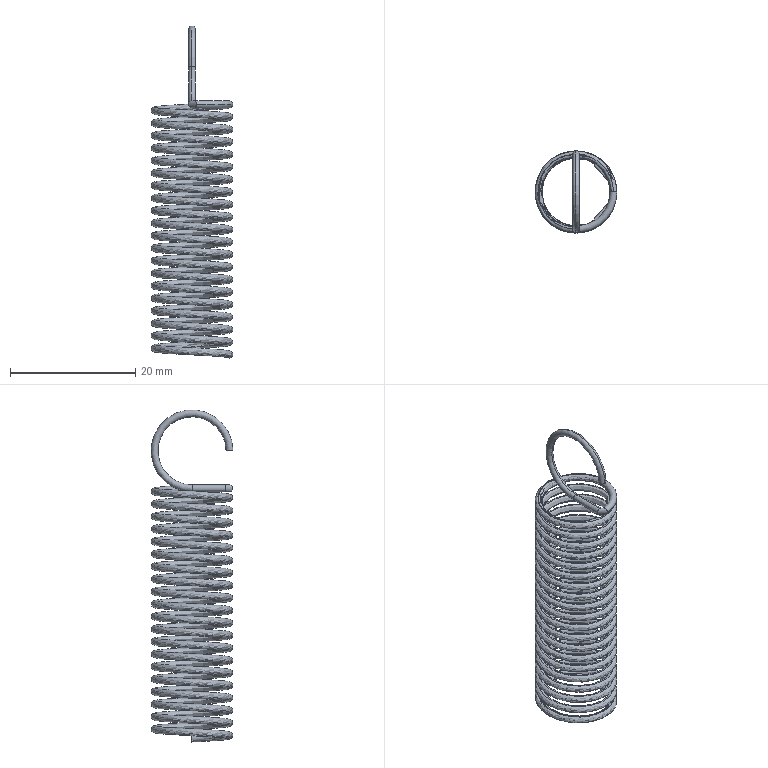Part | STEP file | 0217_Z_AWA12-100 | 1 solid | 11 faces | box 13.1 x 13.1 x 53.1 mm | volume 757.901 mm3 | torus 5 | spline 2 | cylinder 2 | plane 2 | commonest cylinder face diameters 1.1 x2